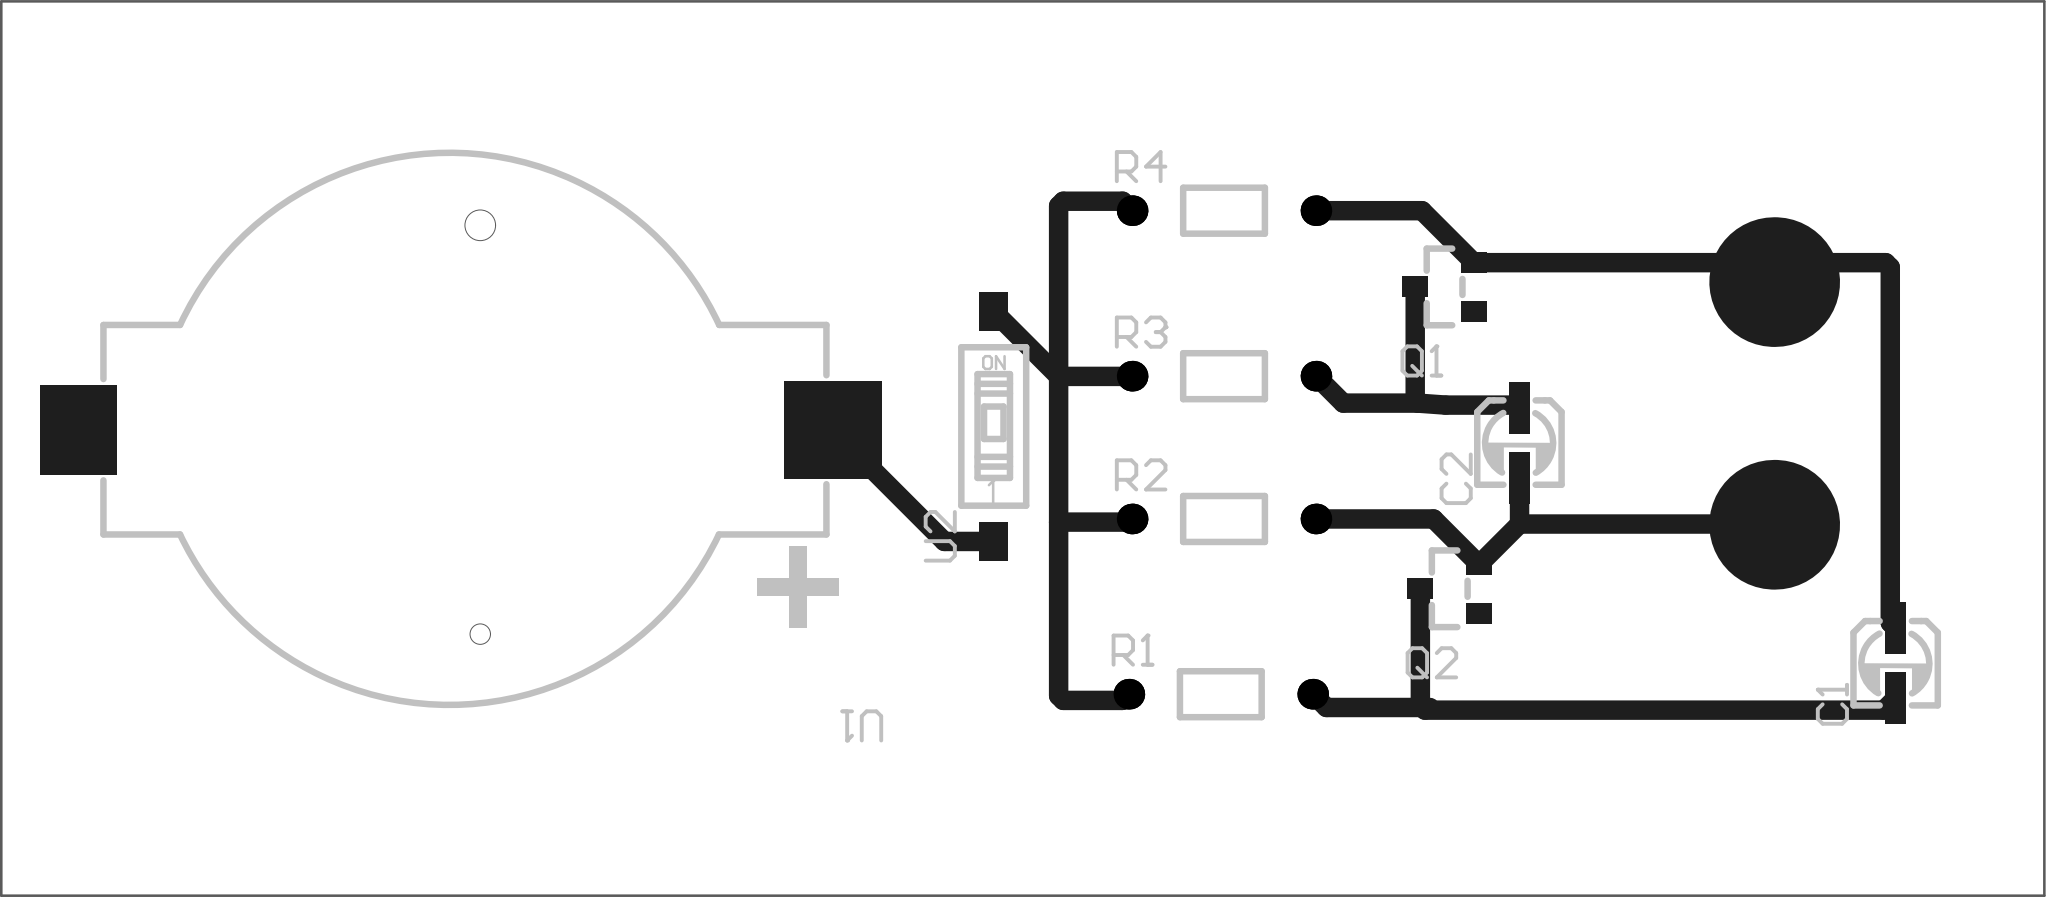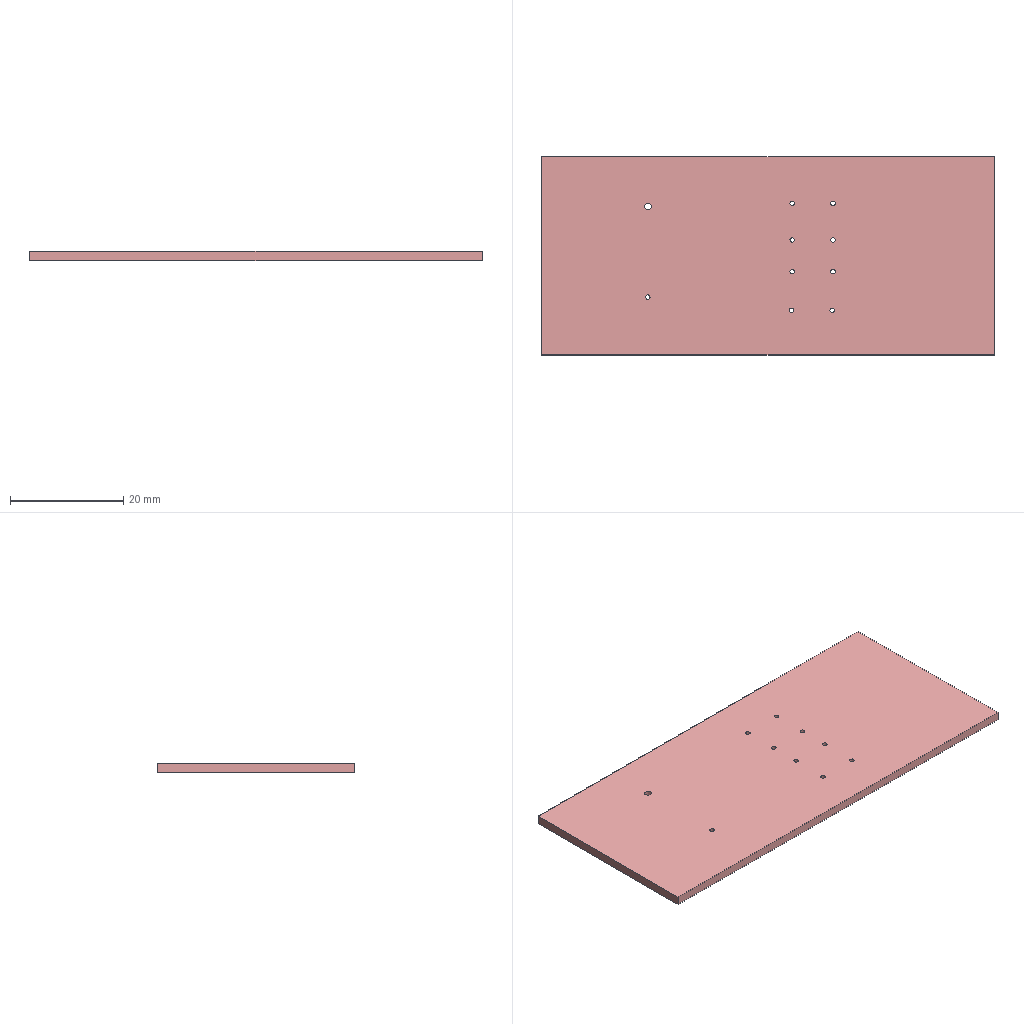Circuit board layout | Altium Designer | box 80 x 35 x 1.6 mm
Layer stack:
# Altium Designer layer stack of  (unit mm; dielectric type: 0 none, 1 core, 2 prepreg, 3 surface material)
index,name,kind,layer,copper_thickness_mm,dielectric_type,dielectric_thickness_mm,dielectric_material,dielectric_constant
0,Top Paste Mask Layer,other,,,,,,
1,Top Silkscreen Layer,other,,,,,,
2,Top Solder Mask Layer,dielectric,,,3,0.01,,3.3
3,Top Layer,copper,Top Layer,0.035,,,,
4,Dielectric1,dielectric,,,3,1.51,FR4,4.5
5,Bottom Layer,copper,Bottom Layer,0.035,,,,
6,Bottom Solder Mask Layer,dielectric,,,3,0.01,,3.3
7,Bottom Silkscreen Layer,other,,,,,,
8,Bottom Paste Mask Layer,other,,,,,,
# drill layer pairs: low layer,high layer
drill_pair,Top Layer,Bottom Layer
Part placement:
Designator,Comment,Layer,Footprint,Center-X(mm),Center-Y(mm),Rotation
R1,10kO,TopLayer,Res_1/8W,123.952,84.085,0
R2,10kO,TopLayer,Res_1/8W,124.079,90.943,0
R3,10kO,TopLayer,Res_1/8W,124.079,96.531,0
R4,10kO,TopLayer,Res_1/8W,124.079,103.008,0
Q1,,TopLayer,S8050_SOT-23,132.715,100.024,0
Q2,,TopLayer,S8050_SOT-23,132.916,88.211,0
C1,10uF,TopLayer,C_Ele_SMD_3x5.4mm,150.382,85.297,90
C2,10uF,TopLayer,C_Ele_SMD_3x5.4mm,135.65,93.933,90
U1,CR2032 battery holder,TopLayer,BAT-SMD_CR2032_C9900016310,93.98,94.436,180
U2,2.54-1P TPGT,TopLayer,SW-SMD_2P-L6.2-W2.5-LS9.4,115.062,94.563,90
Pad and via stacks:
# Altium Designer via and pad stacks of  (unit mm). Each distinct definition once, with the count of objects using it.
# via: kind,start_layer,end_layer,hole_mm,diameter_mm,mode(0 simple;1 top-mid-bottom;2 full stack),diameter_per_layer,count,example_net
# pad: kind,layer,hole_mm,hole_type(0 round;1 square;2 slot),plating,top_size,top_shape(1 round;2 rect;3 octagon;9 rounded rect),mid_size,bottom_size,mode,footprint,size_per_layer,count,example
pad,Multi-Layer,0.8001,0,plated,1.199x1.199,1,1.199x1.199,1.199x1.199,0,Res_1/8W,,8,R1.1
pad,Top Layer,0,0,plated,1x0.8,2,1x0.8,1x0.8,0,S8050_SOT-23,,6,Q1.2
pad,Top Layer,0,0,plated,1.999x0.8001,2,1.999x0.8001,1.999x0.8001,0,C_Ele_SMD_3x5.4mm,,4,C1.1
pad,Top Layer,0,0,plated,3x3.5,2,3x3.5,3x3.5,0,BAT-SMD_CR2032_C9900016310,,1,U1.1
pad,Top Layer,0,0,plated,3.8x3.8,2,3.8x3.8,3.8x3.8,0,BAT-SMD_CR2032_C9900016310,,1,U1.2
pad,Top Layer,0,0,plated,1.1x1.5,2,1.1x1.5,1.1x1.5,0,SW-SMD_2P-L6.2-W2.5-LS9.4,,2,U2.1
pad,Top Layer,0,0,plated,5.08x5.08,1,5.08x5.08,5.08x5.08,0,,,2,1